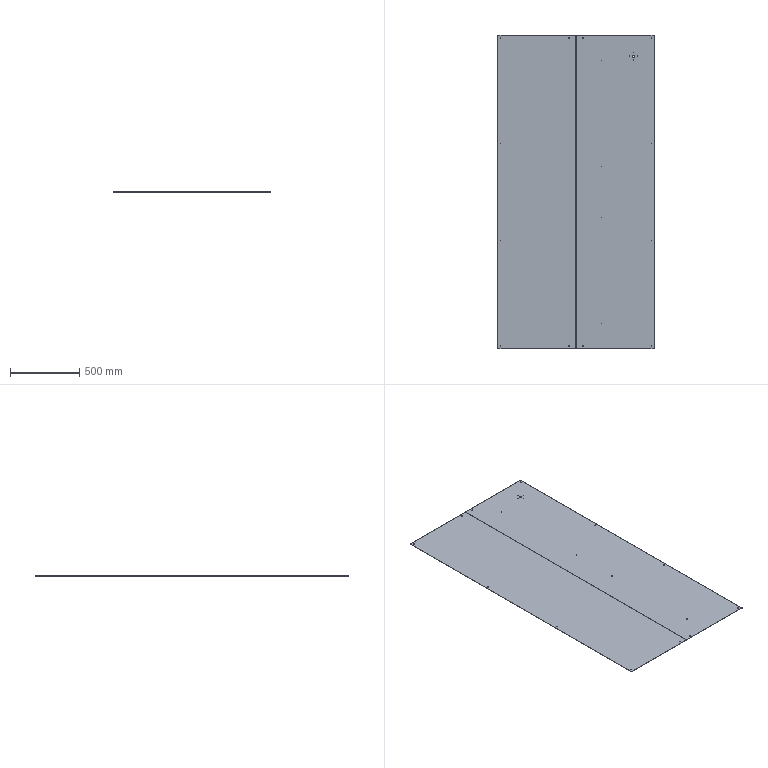Part | STEP file | 2 solids | 58 faces | box 1130 x 2260 x 2 mm | volume 5103955 mm3 | cylinder 46 | plane 12 | commonest cylinder face diameters 6.5 x24 3.3 x8 4.2 x8 4 x4 16 x2